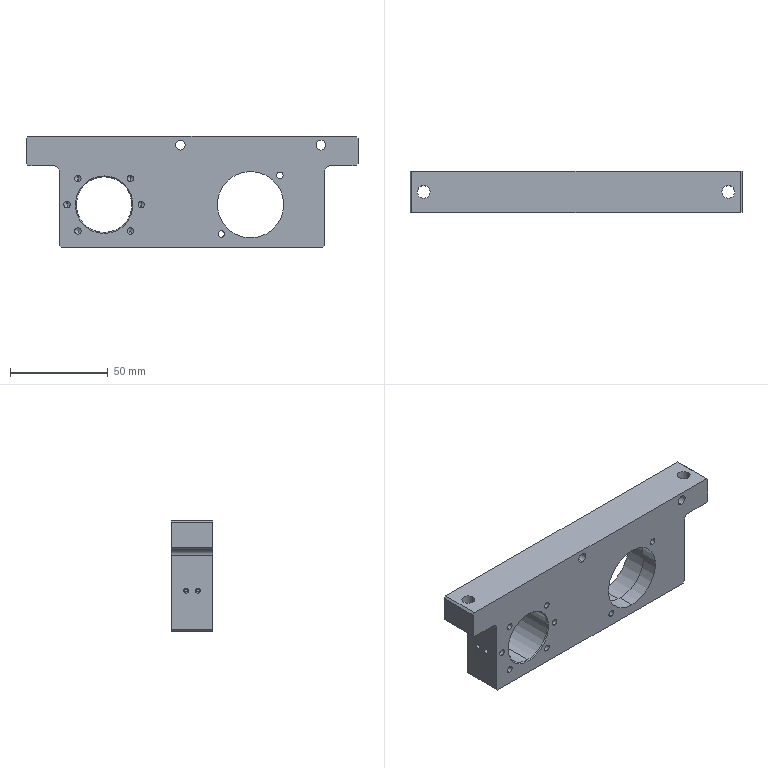Part | STEP file | 1 solid | 78 faces | box 170 x 21 x 57 mm | volume 135678 mm3 | cylinder 39 | cone 20 | plane 19 | commonest cylinder face diameters 3.3 x16 2.5 x4 5 x4 6.5 x4 10 x3 6 x2